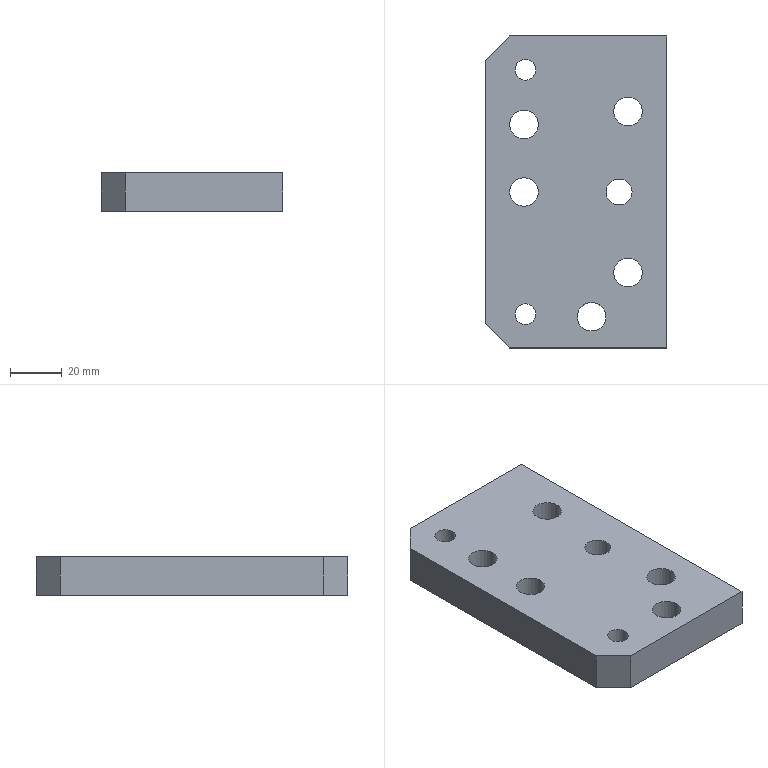Part | STEP file | 1 solid | 16 faces | box 70 x 120 x 15 mm | volume 114867 mm3 | plane 8 | cylinder 8 | commonest cylinder face diameters 11 x5 8 x2 10 x1
STEP:
#1=CARTESIAN_POINT('',(-260.55,50.621,-32.));
#2=VERTEX_POINT('',#1);
#3=CARTESIAN_POINT('',(-260.55,-50.621,-32.));
#4=VERTEX_POINT('',#3);
#5=CARTESIAN_POINT('',(-260.55,47.,-32.));
#6=DIRECTION('',(0.,-1.,0.));
#7=VECTOR('',#6,1.);
#8=LINE('',#5,#7);
#9=EDGE_CURVE('',#2,#4,#8,.T.);
#10=ORIENTED_EDGE('',*,*,#9,.F.);
#11=CARTESIAN_POINT('',(-260.55,50.621,-47.));
#12=VERTEX_POINT('',#11);
#13=CARTESIAN_POINT('',(-260.55,50.621,-32.));
#14=DIRECTION('',(0.,0.,1.));
#15=VECTOR('',#14,1.);
#16=LINE('',#13,#15);
#17=EDGE_CURVE('',#12,#2,#16,.T.);
#18=ORIENTED_EDGE('',*,*,#17,.F.);
#19=CARTESIAN_POINT('',(-260.55,-50.621,-47.));
#20=VERTEX_POINT('',#19);
#21=CARTESIAN_POINT('',(-260.55,0.,-47.));
#22=DIRECTION('',(0.,-1.,0.));
#23=VECTOR('',#22,1.);
#24=LINE('',#21,#23);
#25=EDGE_CURVE('',#12,#20,#24,.T.);
#26=ORIENTED_EDGE('',*,*,#25,.T.);
#27=CARTESIAN_POINT('',(-260.55,-50.621,-32.));
#28=DIRECTION('',(0.,0.,1.));
#29=VECTOR('',#28,1.);
#30=LINE('',#27,#29);
#31=EDGE_CURVE('',#20,#4,#30,.T.);
#32=ORIENTED_EDGE('',*,*,#31,.T.);
#33=EDGE_LOOP('',(#10,#18,#26,#32));
#34=FACE_OUTER_BOUND('',#33,.T.);
#35=CARTESIAN_POINT('',(-260.55,47.,-32.));
#36=DIRECTION('',(1.,0.,0.));
#37=DIRECTION('',(0.,-1.,0.));
#38=AXIS2_PLACEMENT_3D('',#35,#36,#37);
#39=PLANE('',#38);
#40=ADVANCED_FACE('',(#34),#39,.F.);
#41=CARTESIAN_POINT('',(-190.55,-60.,-47.));
#42=VERTEX_POINT('',#41);
#43=CARTESIAN_POINT('',(-190.55,60.,-47.));
#44=VERTEX_POINT('',#43);
#45=CARTESIAN_POINT('',(-190.55,0.,-47.));
#46=DIRECTION('',(0.,1.,0.));
#47=VECTOR('',#46,1.);
#48=LINE('',#45,#47);
#49=EDGE_CURVE('',#42,#44,#48,.T.);
#50=ORIENTED_EDGE('',*,*,#49,.T.);
#51=CARTESIAN_POINT('',(-190.55,60.,-32.));
#52=VERTEX_POINT('',#51);
#53=CARTESIAN_POINT('',(-190.55,60.,-32.));
#54=DIRECTION('',(0.,0.,-1.));
#55=VECTOR('',#54,1.);
#56=LINE('',#53,#55);
#57=EDGE_CURVE('',#52,#44,#56,.T.);
#58=ORIENTED_EDGE('',*,*,#57,.F.);
#59=CARTESIAN_POINT('',(-190.55,-60.,-32.));
#60=VERTEX_POINT('',#59);
#61=CARTESIAN_POINT('',(-190.55,0.,-32.));
#62=DIRECTION('',(0.,1.,0.));
#63=VECTOR('',#62,1.);
#64=LINE('',#61,#63);
#65=EDGE_CURVE('',#60,#52,#64,.T.);
#66=ORIENTED_EDGE('',*,*,#65,.F.);
#67=CARTESIAN_POINT('',(-190.55,-60.,-32.));
#68=DIRECTION('',(0.,0.,-1.));
#69=VECTOR('',#68,1.);
#70=LINE('',#67,#69);
#71=EDGE_CURVE('',#60,#42,#70,.T.);
#72=ORIENTED_EDGE('',*,*,#71,.T.);
#73=EDGE_LOOP('',(#50,#58,#66,#72));
#74=FACE_OUTER_BOUND('',#73,.T.);
#75=CARTESIAN_POINT('',(-190.55,0.,-32.));
#76=DIRECTION('',(-1.,0.,0.));
#77=DIRECTION('',(0.,1.,0.));
#78=AXIS2_PLACEMENT_3D('',#75,#76,#77);
#79=PLANE('',#78);
#80=ADVANCED_FACE('',(#74),#79,.F.);
#81=CARTESIAN_POINT('',(-240.05,26.,-47.));
#82=VERTEX_POINT('',#81);
#83=CARTESIAN_POINT('',(-245.55,26.,-47.));
#84=DIRECTION('',(0.,0.,1.));
#85=DIRECTION('',(1.,0.,0.));
#86=AXIS2_PLACEMENT_3D('',#83,#84,#85);
#87=CIRCLE('',#86,5.5);
#88=EDGE_CURVE('',#82,#82,#87,.T.);
#89=ORIENTED_EDGE('',*,*,#88,.T.);
#90=EDGE_LOOP('',(#89));
#91=FACE_BOUND('',#90,.T.);
#92=CARTESIAN_POINT('',(-240.05,0.,-47.));
#93=VERTEX_POINT('',#92);
#94=CARTESIAN_POINT('',(-245.55,0.,-47.));
#95=DIRECTION('',(0.,0.,-1.));
#96=DIRECTION('',(1.,0.,0.));
#97=AXIS2_PLACEMENT_3D('',#94,#95,#96);
#98=CIRCLE('',#97,5.5);
#99=EDGE_CURVE('',#93,#93,#98,.T.);
#100=ORIENTED_EDGE('',*,*,#99,.F.);
#101=EDGE_LOOP('',(#100));
#102=FACE_BOUND('',#101,.T.);
#103=CARTESIAN_POINT('',(-214.05,-48.,-47.));
#104=VERTEX_POINT('',#103);
#105=CARTESIAN_POINT('',(-219.55,-48.,-47.));
#106=DIRECTION('',(0.,0.,1.));
#107=DIRECTION('',(1.,0.,0.));
#108=AXIS2_PLACEMENT_3D('',#105,#106,#107);
#109=CIRCLE('',#108,5.5);
#110=EDGE_CURVE('',#104,#104,#109,.T.);
#111=ORIENTED_EDGE('',*,*,#110,.T.);
#112=EDGE_LOOP('',(#111));
#113=FACE_BOUND('',#112,.T.);
#114=CARTESIAN_POINT('',(-200.05,31.,-47.));
#115=VERTEX_POINT('',#114);
#116=CARTESIAN_POINT('',(-205.55,31.,-47.));
#117=DIRECTION('',(0.,0.,-1.));
#118=DIRECTION('',(1.,0.,0.));
#119=AXIS2_PLACEMENT_3D('',#116,#117,#118);
#120=CIRCLE('',#119,5.5);
#121=EDGE_CURVE('',#115,#115,#120,.T.);
#122=ORIENTED_EDGE('',*,*,#121,.F.);
#123=EDGE_LOOP('',(#122));
#124=FACE_BOUND('',#123,.T.);
#125=CARTESIAN_POINT('',(-200.05,-31.,-47.));
#126=VERTEX_POINT('',#125);
#127=CARTESIAN_POINT('',(-205.55,-31.,-47.));
#128=DIRECTION('',(0.,0.,1.));
#129=DIRECTION('',(1.,0.,0.));
#130=AXIS2_PLACEMENT_3D('',#127,#128,#129);
#131=CIRCLE('',#130,5.5);
#132=EDGE_CURVE('',#126,#126,#131,.T.);
#133=ORIENTED_EDGE('',*,*,#132,.T.);
#134=EDGE_LOOP('',(#133));
#135=FACE_BOUND('',#134,.T.);
#136=CARTESIAN_POINT('',(-214.,0.,-47.));
#137=VERTEX_POINT('',#136);
#138=CARTESIAN_POINT('',(-209.,0.,-47.));
#139=DIRECTION('',(0.,0.,-1.));
#140=DIRECTION('',(-1.,0.,0.));
#141=AXIS2_PLACEMENT_3D('',#138,#139,#140);
#142=CIRCLE('',#141,5.);
#143=EDGE_CURVE('',#137,#137,#142,.T.);
#144=ORIENTED_EDGE('',*,*,#143,.F.);
#145=EDGE_LOOP('',(#144));
#146=FACE_BOUND('',#145,.T.);
#147=ORIENTED_EDGE('',*,*,#25,.F.);
#148=CARTESIAN_POINT('',(-251.171,60.,-47.));
#149=VERTEX_POINT('',#148);
#150=CARTESIAN_POINT('',(-267.586,43.586,-47.));
#151=DIRECTION('',(-0.7071,-0.7071,0.));
#152=VECTOR('',#151,1.);
#153=LINE('',#150,#152);
#154=EDGE_CURVE('',#149,#12,#153,.T.);
#155=ORIENTED_EDGE('',*,*,#154,.F.);
#156=CARTESIAN_POINT('',(-224.,60.,-47.));
#157=DIRECTION('',(1.,0.,0.));
#158=VECTOR('',#157,1.);
#159=LINE('',#156,#158);
#160=EDGE_CURVE('',#149,#44,#159,.T.);
#161=ORIENTED_EDGE('',*,*,#160,.T.);
#162=ORIENTED_EDGE('',*,*,#49,.F.);
#163=CARTESIAN_POINT('',(-251.171,-60.,-47.));
#164=VERTEX_POINT('',#163);
#165=CARTESIAN_POINT('',(-224.,-60.,-47.));
#166=DIRECTION('',(1.,0.,0.));
#167=VECTOR('',#166,1.);
#168=LINE('',#165,#167);
#169=EDGE_CURVE('',#164,#42,#168,.T.);
#170=ORIENTED_EDGE('',*,*,#169,.F.);
#171=CARTESIAN_POINT('',(-267.586,-43.586,-47.));
#172=DIRECTION('',(-0.7071,0.7071,0.));
#173=VECTOR('',#172,1.);
#174=LINE('',#171,#173);
#175=EDGE_CURVE('',#164,#20,#174,.T.);
#176=ORIENTED_EDGE('',*,*,#175,.T.);
#177=EDGE_LOOP('',(#147,#155,#161,#162,#170,#176));
#178=FACE_BOUND('',#177,.T.);
#179=CARTESIAN_POINT('',(-249.,47.,-47.));
#180=VERTEX_POINT('',#179);
#181=CARTESIAN_POINT('',(-245.,47.,-47.));
#182=DIRECTION('',(0.,0.,-1.));
#183=DIRECTION('',(-1.,0.,0.));
#184=AXIS2_PLACEMENT_3D('',#181,#182,#183);
#185=CIRCLE('',#184,4.);
#186=EDGE_CURVE('',#180,#180,#185,.T.);
#187=ORIENTED_EDGE('',*,*,#186,.F.);
#188=EDGE_LOOP('',(#187));
#189=FACE_BOUND('',#188,.T.);
#190=CARTESIAN_POINT('',(-249.,-47.,-47.));
#191=VERTEX_POINT('',#190);
#192=CARTESIAN_POINT('',(-245.,-47.,-47.));
#193=DIRECTION('',(0.,0.,1.));
#194=DIRECTION('',(-1.,0.,0.));
#195=AXIS2_PLACEMENT_3D('',#192,#193,#194);
#196=CIRCLE('',#195,4.);
#197=EDGE_CURVE('',#191,#191,#196,.T.);
#198=ORIENTED_EDGE('',*,*,#197,.T.);
#199=EDGE_LOOP('',(#198));
#200=FACE_BOUND('',#199,.T.);
#201=CARTESIAN_POINT('',(-224.,0.,-47.));
#202=DIRECTION('',(0.,0.,-1.));
#203=DIRECTION('',(-1.,0.,0.));
#204=AXIS2_PLACEMENT_3D('',#201,#202,#203);
#205=PLANE('',#204);
#206=ADVANCED_FACE('',(#91,#102,#113,#124,#135,#146,#178,#189,#200),#205,.T.);
#207=CARTESIAN_POINT('',(-240.05,26.,-32.));
#208=VERTEX_POINT('',#207);
#209=CARTESIAN_POINT('',(-245.55,26.,-32.));
#210=DIRECTION('',(0.,0.,-1.));
#211=DIRECTION('',(1.,0.,0.));
#212=AXIS2_PLACEMENT_3D('',#209,#210,#211);
#213=CIRCLE('',#212,5.5);
#214=EDGE_CURVE('',#208,#208,#213,.T.);
#215=ORIENTED_EDGE('',*,*,#214,.T.);
#216=EDGE_LOOP('',(#215));
#217=FACE_BOUND('',#216,.T.);
#218=CARTESIAN_POINT('',(-251.05,0.,-32.));
#219=VERTEX_POINT('',#218);
#220=CARTESIAN_POINT('',(-245.55,0.,-32.));
#221=DIRECTION('',(0.,0.,-1.));
#222=DIRECTION('',(-1.,0.,0.));
#223=AXIS2_PLACEMENT_3D('',#220,#221,#222);
#224=CIRCLE('',#223,5.5);
#225=EDGE_CURVE('',#219,#219,#224,.T.);
#226=ORIENTED_EDGE('',*,*,#225,.T.);
#227=EDGE_LOOP('',(#226));
#228=FACE_BOUND('',#227,.T.);
#229=CARTESIAN_POINT('',(-214.05,-48.,-32.));
#230=VERTEX_POINT('',#229);
#231=CARTESIAN_POINT('',(-219.55,-48.,-32.));
#232=DIRECTION('',(0.,0.,-1.));
#233=DIRECTION('',(1.,0.,0.));
#234=AXIS2_PLACEMENT_3D('',#231,#232,#233);
#235=CIRCLE('',#234,5.5);
#236=EDGE_CURVE('',#230,#230,#235,.T.);
#237=ORIENTED_EDGE('',*,*,#236,.T.);
#238=EDGE_LOOP('',(#237));
#239=FACE_BOUND('',#238,.T.);
#240=CARTESIAN_POINT('',(-211.05,31.,-32.));
#241=VERTEX_POINT('',#240);
#242=CARTESIAN_POINT('',(-205.55,31.,-32.));
#243=DIRECTION('',(0.,0.,-1.));
#244=DIRECTION('',(-1.,0.,0.));
#245=AXIS2_PLACEMENT_3D('',#242,#243,#244);
#246=CIRCLE('',#245,5.5);
#247=EDGE_CURVE('',#241,#241,#246,.T.);
#248=ORIENTED_EDGE('',*,*,#247,.T.);
#249=EDGE_LOOP('',(#248));
#250=FACE_BOUND('',#249,.T.);
#251=CARTESIAN_POINT('',(-211.05,-31.,-32.));
#252=VERTEX_POINT('',#251);
#253=CARTESIAN_POINT('',(-205.55,-31.,-32.));
#254=DIRECTION('',(0.,0.,-1.));
#255=DIRECTION('',(-1.,0.,0.));
#256=AXIS2_PLACEMENT_3D('',#253,#254,#255);
#257=CIRCLE('',#256,5.5);
#258=EDGE_CURVE('',#252,#252,#257,.T.);
#259=ORIENTED_EDGE('',*,*,#258,.T.);
#260=EDGE_LOOP('',(#259));
#261=FACE_BOUND('',#260,.T.);
#262=CARTESIAN_POINT('',(-214.,0.,-32.));
#263=VERTEX_POINT('',#262);
#264=CARTESIAN_POINT('',(-209.,0.,-32.));
#265=DIRECTION('',(0.,0.,-1.));
#266=DIRECTION('',(-1.,0.,0.));
#267=AXIS2_PLACEMENT_3D('',#264,#265,#266);
#268=CIRCLE('',#267,5.);
#269=EDGE_CURVE('',#263,#263,#268,.T.);
#270=ORIENTED_EDGE('',*,*,#269,.T.);
#271=EDGE_LOOP('',(#270));
#272=FACE_BOUND('',#271,.T.);
#273=ORIENTED_EDGE('',*,*,#65,.T.);
#274=CARTESIAN_POINT('',(-251.171,60.,-32.));
#275=VERTEX_POINT('',#274);
#276=CARTESIAN_POINT('',(-224.,60.,-32.));
#277=DIRECTION('',(1.,0.,0.));
#278=VECTOR('',#277,1.);
#279=LINE('',#276,#278);
#280=EDGE_CURVE('',#275,#52,#279,.T.);
#281=ORIENTED_EDGE('',*,*,#280,.F.);
#282=CARTESIAN_POINT('',(-258.086,53.086,-32.));
#283=DIRECTION('',(0.7071,0.7071,0.));
#284=VECTOR('',#283,1.);
#285=LINE('',#282,#284);
#286=EDGE_CURVE('',#2,#275,#285,.T.);
#287=ORIENTED_EDGE('',*,*,#286,.F.);
#288=ORIENTED_EDGE('',*,*,#9,.T.);
#289=CARTESIAN_POINT('',(-251.171,-60.,-32.));
#290=VERTEX_POINT('',#289);
#291=CARTESIAN_POINT('',(-258.086,-53.086,-32.));
#292=DIRECTION('',(0.7071,-0.7071,0.));
#293=VECTOR('',#292,1.);
#294=LINE('',#291,#293);
#295=EDGE_CURVE('',#4,#290,#294,.T.);
#296=ORIENTED_EDGE('',*,*,#295,.T.);
#297=CARTESIAN_POINT('',(-224.,-60.,-32.));
#298=DIRECTION('',(1.,0.,0.));
#299=VECTOR('',#298,1.);
#300=LINE('',#297,#299);
#301=EDGE_CURVE('',#290,#60,#300,.T.);
#302=ORIENTED_EDGE('',*,*,#301,.T.);
#303=EDGE_LOOP('',(#273,#281,#287,#288,#296,#302));
#304=FACE_BOUND('',#303,.T.);
#305=CARTESIAN_POINT('',(-249.,47.,-32.));
#306=VERTEX_POINT('',#305);
#307=CARTESIAN_POINT('',(-245.,47.,-32.));
#308=DIRECTION('',(0.,0.,-1.));
#309=DIRECTION('',(-1.,0.,0.));
#310=AXIS2_PLACEMENT_3D('',#307,#308,#309);
#311=CIRCLE('',#310,4.);
#312=EDGE_CURVE('',#306,#306,#311,.T.);
#313=ORIENTED_EDGE('',*,*,#312,.T.);
#314=EDGE_LOOP('',(#313));
#315=FACE_BOUND('',#314,.T.);
#316=CARTESIAN_POINT('',(-249.,-47.,-32.));
#317=VERTEX_POINT('',#316);
#318=CARTESIAN_POINT('',(-245.,-47.,-32.));
#319=DIRECTION('',(0.,0.,1.));
#320=DIRECTION('',(-1.,0.,0.));
#321=AXIS2_PLACEMENT_3D('',#318,#319,#320);
#322=CIRCLE('',#321,4.);
#323=EDGE_CURVE('',#317,#317,#322,.T.);
#324=ORIENTED_EDGE('',*,*,#323,.F.);
#325=EDGE_LOOP('',(#324));
#326=FACE_BOUND('',#325,.T.);
#327=CARTESIAN_POINT('',(-224.,0.,-32.));
#328=DIRECTION('',(0.,0.,-1.));
#329=DIRECTION('',(-1.,0.,0.));
#330=AXIS2_PLACEMENT_3D('',#327,#328,#329);
#331=PLANE('',#330);
#332=ADVANCED_FACE('',(#217,#228,#239,#250,#261,#272,#304,#315,#326),#331,.F.);
#333=ORIENTED_EDGE('',*,*,#143,.T.);
#334=EDGE_LOOP('',(#333));
#335=FACE_BOUND('',#334,.T.);
#336=ORIENTED_EDGE('',*,*,#269,.F.);
#337=EDGE_LOOP('',(#336));
#338=FACE_BOUND('',#337,.T.);
#339=CARTESIAN_POINT('',(-209.,0.,-105.));
#340=DIRECTION('',(0.,0.,1.));
#341=DIRECTION('',(1.,0.,0.));
#342=AXIS2_PLACEMENT_3D('',#339,#340,#341);
#343=CYLINDRICAL_SURFACE('',#342,5.);
#344=ADVANCED_FACE('',(#335,#338),#343,.F.);
#345=ORIENTED_EDGE('',*,*,#280,.T.);
#346=ORIENTED_EDGE('',*,*,#57,.T.);
#347=ORIENTED_EDGE('',*,*,#160,.F.);
#348=CARTESIAN_POINT('',(-251.171,60.,-32.));
#349=DIRECTION('',(0.,0.,-1.));
#350=VECTOR('',#349,1.);
#351=LINE('',#348,#350);
#352=EDGE_CURVE('',#275,#149,#351,.T.);
#353=ORIENTED_EDGE('',*,*,#352,.F.);
#354=EDGE_LOOP('',(#345,#346,#347,#353));
#355=FACE_OUTER_BOUND('',#354,.T.);
#356=CARTESIAN_POINT('',(-224.,60.,-32.));
#357=DIRECTION('',(0.,-1.,0.));
#358=DIRECTION('',(1.,0.,0.));
#359=AXIS2_PLACEMENT_3D('',#356,#357,#358);
#360=PLANE('',#359);
#361=ADVANCED_FACE('',(#355),#360,.F.);
#362=ORIENTED_EDGE('',*,*,#154,.T.);
#363=ORIENTED_EDGE('',*,*,#17,.T.);
#364=ORIENTED_EDGE('',*,*,#286,.T.);
#365=ORIENTED_EDGE('',*,*,#352,.T.);
#366=EDGE_LOOP('',(#362,#363,#364,#365));
#367=FACE_OUTER_BOUND('',#366,.T.);
#368=CARTESIAN_POINT('',(-258.086,53.086,-30.));
#369=DIRECTION('',(0.7071,-0.7071,0.));
#370=DIRECTION('',(0.,0.,1.));
#371=AXIS2_PLACEMENT_3D('',#368,#369,#370);
#372=PLANE('',#371);
#373=ADVANCED_FACE('',(#367),#372,.F.);
#374=ORIENTED_EDGE('',*,*,#186,.T.);
#375=EDGE_LOOP('',(#374));
#376=FACE_BOUND('',#375,.T.);
#377=ORIENTED_EDGE('',*,*,#312,.F.);
#378=EDGE_LOOP('',(#377));
#379=FACE_BOUND('',#378,.T.);
#380=CARTESIAN_POINT('',(-245.,47.,-105.));
#381=DIRECTION('',(0.,0.,1.));
#382=DIRECTION('',(1.,0.,0.));
#383=AXIS2_PLACEMENT_3D('',#380,#381,#382);
#384=CYLINDRICAL_SURFACE('',#383,4.);
#385=ADVANCED_FACE('',(#376,#379),#384,.F.);
#386=ORIENTED_EDGE('',*,*,#301,.F.);
#387=CARTESIAN_POINT('',(-251.171,-60.,-32.));
#388=DIRECTION('',(0.,0.,-1.));
#389=VECTOR('',#388,1.);
#390=LINE('',#387,#389);
#391=EDGE_CURVE('',#290,#164,#390,.T.);
#392=ORIENTED_EDGE('',*,*,#391,.T.);
#393=ORIENTED_EDGE('',*,*,#169,.T.);
#394=ORIENTED_EDGE('',*,*,#71,.F.);
#395=EDGE_LOOP('',(#386,#392,#393,#394));
#396=FACE_OUTER_BOUND('',#395,.T.);
#397=CARTESIAN_POINT('',(-224.,-60.,-32.));
#398=DIRECTION('',(0.,1.,0.));
#399=DIRECTION('',(1.,0.,0.));
#400=AXIS2_PLACEMENT_3D('',#397,#398,#399);
#401=PLANE('',#400);
#402=ADVANCED_FACE('',(#396),#401,.F.);
#403=ORIENTED_EDGE('',*,*,#175,.F.);
#404=ORIENTED_EDGE('',*,*,#391,.F.);
#405=ORIENTED_EDGE('',*,*,#295,.F.);
#406=ORIENTED_EDGE('',*,*,#31,.F.);
#407=EDGE_LOOP('',(#403,#404,#405,#406));
#408=FACE_OUTER_BOUND('',#407,.T.);
#409=CARTESIAN_POINT('',(-258.086,-53.086,-30.));
#410=DIRECTION('',(0.7071,0.7071,0.));
#411=DIRECTION('',(0.,0.,1.));
#412=AXIS2_PLACEMENT_3D('',#409,#410,#411);
#413=PLANE('',#412);
#414=ADVANCED_FACE('',(#408),#413,.F.);
#415=ORIENTED_EDGE('',*,*,#197,.F.);
#416=EDGE_LOOP('',(#415));
#417=FACE_BOUND('',#416,.T.);
#418=ORIENTED_EDGE('',*,*,#323,.T.);
#419=EDGE_LOOP('',(#418));
#420=FACE_BOUND('',#419,.T.);
#421=CARTESIAN_POINT('',(-245.,-47.,-105.));
#422=DIRECTION('',(0.,0.,1.));
#423=DIRECTION('',(1.,0.,0.));
#424=AXIS2_PLACEMENT_3D('',#421,#422,#423);
#425=CYLINDRICAL_SURFACE('',#424,4.);
#426=ADVANCED_FACE('',(#417,#420),#425,.F.);
#427=ORIENTED_EDGE('',*,*,#132,.F.);
#428=EDGE_LOOP('',(#427));
#429=FACE_BOUND('',#428,.T.);
#430=ORIENTED_EDGE('',*,*,#258,.F.);
#431=EDGE_LOOP('',(#430));
#432=FACE_BOUND('',#431,.T.);
#433=CARTESIAN_POINT('',(-205.55,-31.,-47.));
#434=DIRECTION('',(0.,0.,1.));
#435=DIRECTION('',(1.,0.,0.));
#436=AXIS2_PLACEMENT_3D('',#433,#434,#435);
#437=CYLINDRICAL_SURFACE('',#436,5.5);
#438=ADVANCED_FACE('',(#429,#432),#437,.F.);
#439=ORIENTED_EDGE('',*,*,#121,.T.);
#440=EDGE_LOOP('',(#439));
#441=FACE_BOUND('',#440,.T.);
#442=ORIENTED_EDGE('',*,*,#247,.F.);
#443=EDGE_LOOP('',(#442));
#444=FACE_BOUND('',#443,.T.);
#445=CARTESIAN_POINT('',(-205.55,31.,-47.));
#446=DIRECTION('',(0.,0.,1.));
#447=DIRECTION('',(1.,0.,0.));
#448=AXIS2_PLACEMENT_3D('',#445,#446,#447);
#449=CYLINDRICAL_SURFACE('',#448,5.5);
#450=ADVANCED_FACE('',(#441,#444),#449,.F.);
#451=ORIENTED_EDGE('',*,*,#236,.F.);
#452=EDGE_LOOP('',(#451));
#453=FACE_BOUND('',#452,.T.);
#454=ORIENTED_EDGE('',*,*,#110,.F.);
#455=EDGE_LOOP('',(#454));
#456=FACE_BOUND('',#455,.T.);
#457=CARTESIAN_POINT('',(-219.55,-48.,-47.));
#458=DIRECTION('',(0.,0.,1.));
#459=DIRECTION('',(1.,0.,0.));
#460=AXIS2_PLACEMENT_3D('',#457,#458,#459);
#461=CYLINDRICAL_SURFACE('',#460,5.5);
#462=ADVANCED_FACE('',(#453,#456),#461,.F.);
#463=ORIENTED_EDGE('',*,*,#99,.T.);
#464=EDGE_LOOP('',(#463));
#465=FACE_BOUND('',#464,.T.);
#466=ORIENTED_EDGE('',*,*,#225,.F.);
#467=EDGE_LOOP('',(#466));
#468=FACE_BOUND('',#467,.T.);
#469=CARTESIAN_POINT('',(-245.55,0.,-47.));
#470=DIRECTION('',(0.,0.,1.));
#471=DIRECTION('',(1.,0.,0.));
#472=AXIS2_PLACEMENT_3D('',#469,#470,#471);
#473=CYLINDRICAL_SURFACE('',#472,5.5);
#474=ADVANCED_FACE('',(#465,#468),#473,.F.);
#475=ORIENTED_EDGE('',*,*,#214,.F.);
#476=EDGE_LOOP('',(#475));
#477=FACE_BOUND('',#476,.T.);
#478=ORIENTED_EDGE('',*,*,#88,.F.);
#479=EDGE_LOOP('',(#478));
#480=FACE_BOUND('',#479,.T.);
#481=CARTESIAN_POINT('',(-245.55,26.,-47.));
#482=DIRECTION('',(0.,0.,1.));
#483=DIRECTION('',(1.,0.,0.));
#484=AXIS2_PLACEMENT_3D('',#481,#482,#483);
#485=CYLINDRICAL_SURFACE('',#484,5.5);
#486=ADVANCED_FACE('',(#477,#480),#485,.F.);
#487=CLOSED_SHELL('',(#40,#80,#206,#332,#344,#361,#373,#385,#402,#414,#426,#438,#450,#462,#474,#486));
#488=MANIFOLD_SOLID_BREP('',#487);
#489=(LENGTH_UNIT()NAMED_UNIT(*)SI_UNIT(.MILLI.,.METRE.));
#490=UNCERTAINTY_MEASURE_WITH_UNIT(LENGTH_MEASURE(0.00002),#489,'','');
#491=(NAMED_UNIT(*)PLANE_ANGLE_UNIT()SI_UNIT($,.RADIAN.));
#492=PLANE_ANGLE_MEASURE_WITH_UNIT(PLANE_ANGLE_MEASURE(0.01745),#491);
#493=DIMENSIONAL_EXPONENTS(0.,0.,0.,0.,0.,0.,0.);
#494=(CONVERSION_BASED_UNIT('DEGREE',#492)NAMED_UNIT(#493)PLANE_ANGLE_UNIT());
#495=(NAMED_UNIT(*)SI_UNIT($,.STERADIAN.)SOLID_ANGLE_UNIT());
#496=(GEOMETRIC_REPRESENTATION_CONTEXT(3)GLOBAL_UNCERTAINTY_ASSIGNED_CONTEXT((#490))GLOBAL_UNIT_ASSIGNED_CONTEXT((#489,#494,#495))REPRESENTATION_CONTEXT('',''));
#497=ADVANCED_BREP_SHAPE_REPRESENTATION('',(#488),#496);